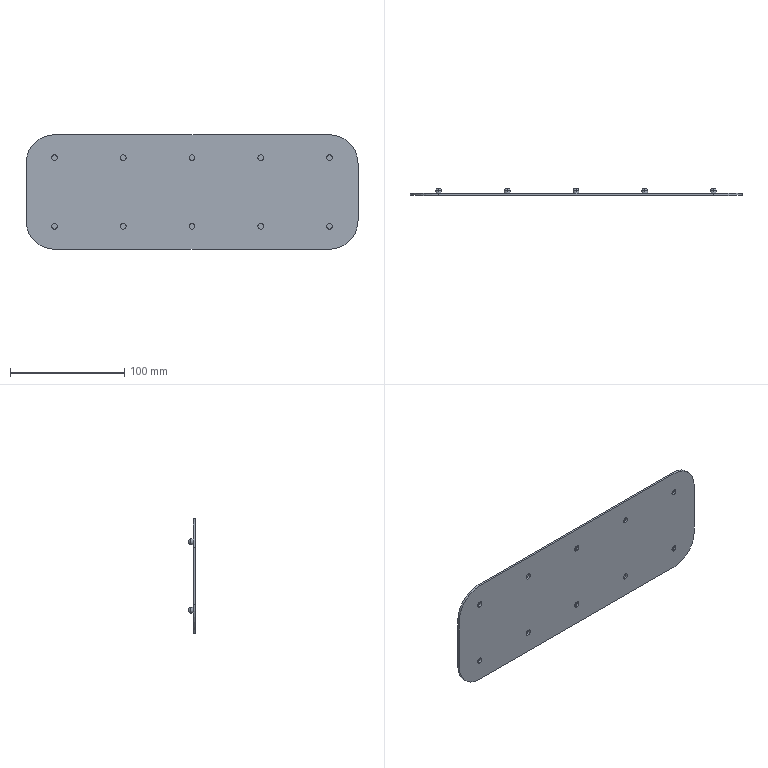Part | SolidWorks | features Fillet 10, FlatPattern 1, ICE 1, SMBaseFlange 1, SheetMetal 1 | 11 solids | 90 faces | box 290 x 6 x 100 mm | volume 57219 mm3 | cylinder 44 | plane 26 | torus 20 | commonest cylinder face diameters 5 x40 50 x4